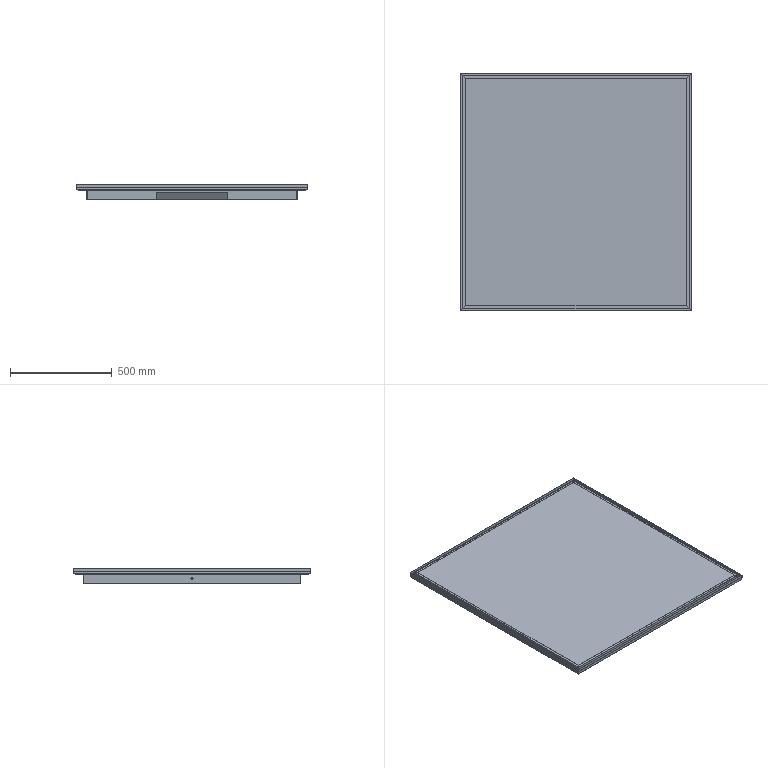Part | 7 solids | 282 faces | box 1140 x 1170 x 75 mm | volume 29962206 mm3 | plane 148 | cylinder 122 | spline 12 | commonest cylinder face diameters 4.2 x80 11 x14 0.4 x11 2.4 x11 10 x6